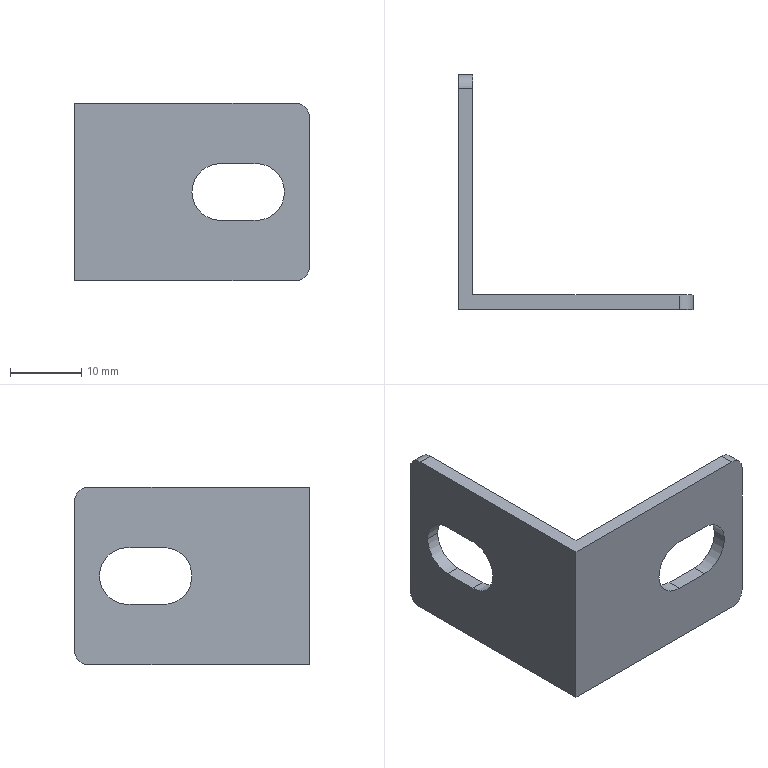Part | SolidWorks | features ICE 2, Extrusion 1, Fillet 1 | 1 solid | 22 faces | box 33 x 33 x 25 mm | volume 2832 mm3 | plane 12 | cylinder 10 | commonest cylinder face diameters 8 x6 4 x4
STEP:
#1=CARTESIAN_POINT('',(0.,29.5,12.5));
#2=VERTEX_POINT('',#1);
#3=CARTESIAN_POINT('',(0.,25.5,16.5));
#4=VERTEX_POINT('',#3);
#5=CARTESIAN_POINT('',(0.,25.5,12.5));
#6=DIRECTION('',(1.,0.,0.));
#7=DIRECTION('',(0.,1.,0.));
#8=AXIS2_PLACEMENT_3D('',#5,#6,#7);
#9=CIRCLE('',#8,4.);
#10=EDGE_CURVE('',#2,#4,#9,.T.);
#11=ORIENTED_EDGE('',*,*,#10,.F.);
#12=CARTESIAN_POINT('',(2.,29.5,12.5));
#13=VERTEX_POINT('',#12);
#14=CARTESIAN_POINT('',(0.,29.5,12.5));
#15=DIRECTION('',(1.,0.,0.));
#16=VECTOR('',#15,1000.);
#17=LINE('',#14,#16);
#18=EDGE_CURVE('',#2,#13,#17,.T.);
#19=ORIENTED_EDGE('',*,*,#18,.T.);
#20=CARTESIAN_POINT('',(2.,25.5,16.5));
#21=VERTEX_POINT('',#20);
#22=CARTESIAN_POINT('',(2.,25.5,12.5));
#23=DIRECTION('',(1.,0.,0.));
#24=DIRECTION('',(0.,1.,0.));
#25=AXIS2_PLACEMENT_3D('',#22,#23,#24);
#26=CIRCLE('',#25,4.);
#27=EDGE_CURVE('',#13,#21,#26,.T.);
#28=ORIENTED_EDGE('',*,*,#27,.T.);
#29=CARTESIAN_POINT('',(0.,25.5,16.5));
#30=DIRECTION('',(1.,0.,0.));
#31=VECTOR('',#30,1000.);
#32=LINE('',#29,#31);
#33=EDGE_CURVE('',#4,#21,#32,.T.);
#34=ORIENTED_EDGE('',*,*,#33,.F.);
#35=EDGE_LOOP('',(#11,#19,#28,#34));
#36=FACE_OUTER_BOUND('',#35,.T.);
#37=CARTESIAN_POINT('',(0.,25.5,12.5));
#38=DIRECTION('',(1.,0.,0.));
#39=DIRECTION('',(0.,1.,0.));
#40=AXIS2_PLACEMENT_3D('',#37,#38,#39);
#41=CYLINDRICAL_SURFACE('',#40,4.);
#42=ADVANCED_FACE('',(#36),#41,.F.);
#43=CARTESIAN_POINT('',(16.5,0.,12.5));
#44=VERTEX_POINT('',#43);
#45=CARTESIAN_POINT('',(20.5,0.,16.5));
#46=VERTEX_POINT('',#45);
#47=CARTESIAN_POINT('',(20.5,0.,12.5));
#48=DIRECTION('',(0.,1.,0.));
#49=DIRECTION('',(-1.,0.,0.));
#50=AXIS2_PLACEMENT_3D('',#47,#48,#49);
#51=CIRCLE('',#50,4.);
#52=EDGE_CURVE('',#44,#46,#51,.T.);
#53=ORIENTED_EDGE('',*,*,#52,.F.);
#54=CARTESIAN_POINT('',(16.5,2.,12.5));
#55=VERTEX_POINT('',#54);
#56=CARTESIAN_POINT('',(16.5,0.,12.5));
#57=DIRECTION('',(0.,1.,0.));
#58=VECTOR('',#57,1000.);
#59=LINE('',#56,#58);
#60=EDGE_CURVE('',#44,#55,#59,.T.);
#61=ORIENTED_EDGE('',*,*,#60,.T.);
#62=CARTESIAN_POINT('',(20.5,2.,16.5));
#63=VERTEX_POINT('',#62);
#64=CARTESIAN_POINT('',(20.5,2.,12.5));
#65=DIRECTION('',(0.,1.,0.));
#66=DIRECTION('',(-1.,0.,0.));
#67=AXIS2_PLACEMENT_3D('',#64,#65,#66);
#68=CIRCLE('',#67,4.);
#69=EDGE_CURVE('',#55,#63,#68,.T.);
#70=ORIENTED_EDGE('',*,*,#69,.T.);
#71=CARTESIAN_POINT('',(20.5,0.,16.5));
#72=DIRECTION('',(0.,1.,0.));
#73=VECTOR('',#72,1000.);
#74=LINE('',#71,#73);
#75=EDGE_CURVE('',#46,#63,#74,.T.);
#76=ORIENTED_EDGE('',*,*,#75,.F.);
#77=EDGE_LOOP('',(#53,#61,#70,#76));
#78=FACE_OUTER_BOUND('',#77,.T.);
#79=CARTESIAN_POINT('',(20.5,0.,12.5));
#80=DIRECTION('',(0.,1.,0.));
#81=DIRECTION('',(-1.,0.,0.));
#82=AXIS2_PLACEMENT_3D('',#79,#80,#81);
#83=CYLINDRICAL_SURFACE('',#82,4.);
#84=ADVANCED_FACE('',(#78),#83,.F.);
#85=CARTESIAN_POINT('',(0.,20.5,8.5));
#86=VERTEX_POINT('',#85);
#87=CARTESIAN_POINT('',(0.,25.5,8.5));
#88=VERTEX_POINT('',#87);
#89=CARTESIAN_POINT('',(0.,25.5,8.5));
#90=DIRECTION('',(0.,1.,0.));
#91=VECTOR('',#90,1000.);
#92=LINE('',#89,#91);
#93=EDGE_CURVE('',#86,#88,#92,.T.);
#94=ORIENTED_EDGE('',*,*,#93,.T.);
#95=CARTESIAN_POINT('',(0.,25.5,12.5));
#96=DIRECTION('',(1.,0.,0.));
#97=DIRECTION('',(0.,1.,0.));
#98=AXIS2_PLACEMENT_3D('',#95,#96,#97);
#99=CIRCLE('',#98,4.);
#100=EDGE_CURVE('',#88,#2,#99,.T.);
#101=ORIENTED_EDGE('',*,*,#100,.T.);
#102=ORIENTED_EDGE('',*,*,#10,.T.);
#103=CARTESIAN_POINT('',(0.,20.5,16.5));
#104=VERTEX_POINT('',#103);
#105=CARTESIAN_POINT('',(0.,25.5,16.5));
#106=DIRECTION('',(0.,-1.,0.));
#107=VECTOR('',#106,1000.);
#108=LINE('',#105,#107);
#109=EDGE_CURVE('',#4,#104,#108,.T.);
#110=ORIENTED_EDGE('',*,*,#109,.T.);
#111=CARTESIAN_POINT('',(0.,20.5,12.5));
#112=DIRECTION('',(1.,0.,0.));
#113=DIRECTION('',(0.,1.,0.));
#114=AXIS2_PLACEMENT_3D('',#111,#112,#113);
#115=CIRCLE('',#114,4.);
#116=EDGE_CURVE('',#104,#86,#115,.T.);
#117=ORIENTED_EDGE('',*,*,#116,.T.);
#118=EDGE_LOOP('',(#94,#101,#102,#110,#117));
#119=FACE_BOUND('',#118,.T.);
#120=CARTESIAN_POINT('',(0.,33.,23.));
#121=VERTEX_POINT('',#120);
#122=CARTESIAN_POINT('',(0.,33.,2.));
#123=VERTEX_POINT('',#122);
#124=CARTESIAN_POINT('',(0.,33.,25.));
#125=DIRECTION('',(0.,0.,-1.));
#126=VECTOR('',#125,1000.);
#127=LINE('',#124,#126);
#128=EDGE_CURVE('',#121,#123,#127,.T.);
#129=ORIENTED_EDGE('',*,*,#128,.T.);
#130=CARTESIAN_POINT('',(0.,31.,0.));
#131=VERTEX_POINT('',#130);
#132=CARTESIAN_POINT('',(0.,31.,2.));
#133=DIRECTION('',(-1.,0.,0.));
#134=DIRECTION('',(0.,1.,0.));
#135=AXIS2_PLACEMENT_3D('',#132,#133,#134);
#136=CIRCLE('',#135,2.);
#137=EDGE_CURVE('',#123,#131,#136,.T.);
#138=ORIENTED_EDGE('',*,*,#137,.T.);
#139=CARTESIAN_POINT('',(0.,0.,0.));
#140=VERTEX_POINT('',#139);
#141=CARTESIAN_POINT('',(0.,33.,0.));
#142=DIRECTION('',(0.,-1.,0.));
#143=VECTOR('',#142,1000.);
#144=LINE('',#141,#143);
#145=EDGE_CURVE('',#131,#140,#144,.T.);
#146=ORIENTED_EDGE('',*,*,#145,.T.);
#147=CARTESIAN_POINT('',(0.,0.,25.));
#148=VERTEX_POINT('',#147);
#149=CARTESIAN_POINT('',(0.,0.,25.));
#150=DIRECTION('',(0.,0.,-1.));
#151=VECTOR('',#150,1000.);
#152=LINE('',#149,#151);
#153=EDGE_CURVE('',#148,#140,#152,.T.);
#154=ORIENTED_EDGE('',*,*,#153,.F.);
#155=CARTESIAN_POINT('',(0.,31.,25.));
#156=VERTEX_POINT('',#155);
#157=CARTESIAN_POINT('',(0.,33.,25.));
#158=DIRECTION('',(0.,-1.,0.));
#159=VECTOR('',#158,1000.);
#160=LINE('',#157,#159);
#161=EDGE_CURVE('',#156,#148,#160,.T.);
#162=ORIENTED_EDGE('',*,*,#161,.F.);
#163=CARTESIAN_POINT('',(0.,31.,23.));
#164=DIRECTION('',(-1.,0.,0.));
#165=DIRECTION('',(0.,1.,0.));
#166=AXIS2_PLACEMENT_3D('',#163,#164,#165);
#167=CIRCLE('',#166,2.);
#168=EDGE_CURVE('',#156,#121,#167,.T.);
#169=ORIENTED_EDGE('',*,*,#168,.T.);
#170=EDGE_LOOP('',(#129,#138,#146,#154,#162,#169));
#171=FACE_OUTER_BOUND('',#170,.T.);
#172=CARTESIAN_POINT('',(0.,33.,25.));
#173=DIRECTION('',(1.,0.,0.));
#174=DIRECTION('',(0.,1.,0.));
#175=AXIS2_PLACEMENT_3D('',#172,#173,#174);
#176=PLANE('',#175);
#177=ADVANCED_FACE('',(#119,#171),#176,.F.);
#178=CARTESIAN_POINT('',(25.5,0.,8.5));
#179=VERTEX_POINT('',#178);
#180=CARTESIAN_POINT('',(20.5,0.,8.5));
#181=VERTEX_POINT('',#180);
#182=CARTESIAN_POINT('',(20.5,0.,8.5));
#183=DIRECTION('',(-1.,0.,0.));
#184=VECTOR('',#183,1000.);
#185=LINE('',#182,#184);
#186=EDGE_CURVE('',#179,#181,#185,.T.);
#187=ORIENTED_EDGE('',*,*,#186,.T.);
#188=CARTESIAN_POINT('',(20.5,0.,12.5));
#189=DIRECTION('',(0.,1.,0.));
#190=DIRECTION('',(-1.,0.,0.));
#191=AXIS2_PLACEMENT_3D('',#188,#189,#190);
#192=CIRCLE('',#191,4.);
#193=EDGE_CURVE('',#181,#44,#192,.T.);
#194=ORIENTED_EDGE('',*,*,#193,.T.);
#195=ORIENTED_EDGE('',*,*,#52,.T.);
#196=CARTESIAN_POINT('',(25.5,0.,16.5));
#197=VERTEX_POINT('',#196);
#198=CARTESIAN_POINT('',(20.5,0.,16.5));
#199=DIRECTION('',(1.,0.,0.));
#200=VECTOR('',#199,1000.);
#201=LINE('',#198,#200);
#202=EDGE_CURVE('',#46,#197,#201,.T.);
#203=ORIENTED_EDGE('',*,*,#202,.T.);
#204=CARTESIAN_POINT('',(25.5,0.,12.5));
#205=DIRECTION('',(0.,1.,0.));
#206=DIRECTION('',(-1.,0.,0.));
#207=AXIS2_PLACEMENT_3D('',#204,#205,#206);
#208=CIRCLE('',#207,4.);
#209=EDGE_CURVE('',#197,#179,#208,.T.);
#210=ORIENTED_EDGE('',*,*,#209,.T.);
#211=EDGE_LOOP('',(#187,#194,#195,#203,#210));
#212=FACE_BOUND('',#211,.T.);
#213=CARTESIAN_POINT('',(33.,0.,23.));
#214=VERTEX_POINT('',#213);
#215=CARTESIAN_POINT('',(33.,0.,2.));
#216=VERTEX_POINT('',#215);
#217=CARTESIAN_POINT('',(33.,0.,25.));
#218=DIRECTION('',(0.,0.,-1.));
#219=VECTOR('',#218,1000.);
#220=LINE('',#217,#219);
#221=EDGE_CURVE('',#214,#216,#220,.T.);
#222=ORIENTED_EDGE('',*,*,#221,.F.);
#223=CARTESIAN_POINT('',(31.,0.,25.));
#224=VERTEX_POINT('',#223);
#225=CARTESIAN_POINT('',(31.,0.,23.));
#226=DIRECTION('',(0.,-1.,0.));
#227=DIRECTION('',(0.,0.,1.));
#228=AXIS2_PLACEMENT_3D('',#225,#226,#227);
#229=CIRCLE('',#228,2.);
#230=EDGE_CURVE('',#214,#224,#229,.T.);
#231=ORIENTED_EDGE('',*,*,#230,.T.);
#232=CARTESIAN_POINT('',(0.,0.,25.));
#233=DIRECTION('',(1.,0.,0.));
#234=VECTOR('',#233,1000.);
#235=LINE('',#232,#234);
#236=EDGE_CURVE('',#148,#224,#235,.T.);
#237=ORIENTED_EDGE('',*,*,#236,.F.);
#238=ORIENTED_EDGE('',*,*,#153,.T.);
#239=CARTESIAN_POINT('',(31.,0.,0.));
#240=VERTEX_POINT('',#239);
#241=CARTESIAN_POINT('',(0.,0.,0.));
#242=DIRECTION('',(1.,0.,0.));
#243=VECTOR('',#242,1000.);
#244=LINE('',#241,#243);
#245=EDGE_CURVE('',#140,#240,#244,.T.);
#246=ORIENTED_EDGE('',*,*,#245,.T.);
#247=CARTESIAN_POINT('',(31.,0.,2.));
#248=DIRECTION('',(0.,-1.,0.));
#249=DIRECTION('',(0.,0.,1.));
#250=AXIS2_PLACEMENT_3D('',#247,#248,#249);
#251=CIRCLE('',#250,2.);
#252=EDGE_CURVE('',#240,#216,#251,.T.);
#253=ORIENTED_EDGE('',*,*,#252,.T.);
#254=EDGE_LOOP('',(#222,#231,#237,#238,#246,#253));
#255=FACE_OUTER_BOUND('',#254,.T.);
#256=CARTESIAN_POINT('',(0.,0.,25.));
#257=DIRECTION('',(0.,1.,0.));
#258=DIRECTION('',(0.,0.,1.));
#259=AXIS2_PLACEMENT_3D('',#256,#257,#258);
#260=PLANE('',#259);
#261=ADVANCED_FACE('',(#212,#255),#260,.F.);
#262=CARTESIAN_POINT('',(33.,2.,23.));
#263=VERTEX_POINT('',#262);
#264=CARTESIAN_POINT('',(33.,2.,2.));
#265=VERTEX_POINT('',#264);
#266=CARTESIAN_POINT('',(33.,2.,25.));
#267=DIRECTION('',(0.,0.,-1.));
#268=VECTOR('',#267,1000.);
#269=LINE('',#266,#268);
#270=EDGE_CURVE('',#263,#265,#269,.T.);
#271=ORIENTED_EDGE('',*,*,#270,.F.);
#272=CARTESIAN_POINT('',(33.,0.,23.));
#273=DIRECTION('',(0.,-1.,0.));
#274=VECTOR('',#273,1000.);
#275=LINE('',#272,#274);
#276=EDGE_CURVE('',#263,#214,#275,.T.);
#277=ORIENTED_EDGE('',*,*,#276,.T.);
#278=ORIENTED_EDGE('',*,*,#221,.T.);
#279=CARTESIAN_POINT('',(33.,0.,2.));
#280=DIRECTION('',(0.,1.,0.));
#281=VECTOR('',#280,1000.);
#282=LINE('',#279,#281);
#283=EDGE_CURVE('',#216,#265,#282,.T.);
#284=ORIENTED_EDGE('',*,*,#283,.T.);
#285=EDGE_LOOP('',(#271,#277,#278,#284));
#286=FACE_OUTER_BOUND('',#285,.T.);
#287=CARTESIAN_POINT('',(33.,0.,25.));
#288=DIRECTION('',(-1.,0.,0.));
#289=DIRECTION('',(0.,0.,1.));
#290=AXIS2_PLACEMENT_3D('',#287,#288,#289);
#291=PLANE('',#290);
#292=ADVANCED_FACE('',(#286),#291,.F.);
#293=CARTESIAN_POINT('',(25.5,2.,16.5));
#294=VERTEX_POINT('',#293);
#295=CARTESIAN_POINT('',(20.5,2.,16.5));
#296=DIRECTION('',(1.,0.,0.));
#297=VECTOR('',#296,1000.);
#298=LINE('',#295,#297);
#299=EDGE_CURVE('',#63,#294,#298,.T.);
#300=ORIENTED_EDGE('',*,*,#299,.F.);
#301=ORIENTED_EDGE('',*,*,#69,.F.);
#302=CARTESIAN_POINT('',(20.5,2.,8.5));
#303=VERTEX_POINT('',#302);
#304=CARTESIAN_POINT('',(20.5,2.,12.5));
#305=DIRECTION('',(0.,1.,0.));
#306=DIRECTION('',(-1.,0.,0.));
#307=AXIS2_PLACEMENT_3D('',#304,#305,#306);
#308=CIRCLE('',#307,4.);
#309=EDGE_CURVE('',#303,#55,#308,.T.);
#310=ORIENTED_EDGE('',*,*,#309,.F.);
#311=CARTESIAN_POINT('',(25.5,2.,8.5));
#312=VERTEX_POINT('',#311);
#313=CARTESIAN_POINT('',(20.5,2.,8.5));
#314=DIRECTION('',(-1.,0.,0.));
#315=VECTOR('',#314,1000.);
#316=LINE('',#313,#315);
#317=EDGE_CURVE('',#312,#303,#316,.T.);
#318=ORIENTED_EDGE('',*,*,#317,.F.);
#319=CARTESIAN_POINT('',(25.5,2.,12.5));
#320=DIRECTION('',(0.,1.,0.));
#321=DIRECTION('',(-1.,0.,0.));
#322=AXIS2_PLACEMENT_3D('',#319,#320,#321);
#323=CIRCLE('',#322,4.);
#324=EDGE_CURVE('',#294,#312,#323,.T.);
#325=ORIENTED_EDGE('',*,*,#324,.F.);
#326=EDGE_LOOP('',(#300,#301,#310,#318,#325));
#327=FACE_BOUND('',#326,.T.);
#328=CARTESIAN_POINT('',(31.,2.,25.));
#329=VERTEX_POINT('',#328);
#330=CARTESIAN_POINT('',(2.,2.,25.));
#331=VERTEX_POINT('',#330);
#332=CARTESIAN_POINT('',(33.,2.,25.));
#333=DIRECTION('',(-1.,0.,0.));
#334=VECTOR('',#333,1000.);
#335=LINE('',#332,#334);
#336=EDGE_CURVE('',#329,#331,#335,.T.);
#337=ORIENTED_EDGE('',*,*,#336,.F.);
#338=CARTESIAN_POINT('',(31.,2.,23.));
#339=DIRECTION('',(0.,1.,0.));
#340=DIRECTION('',(1.,0.,0.));
#341=AXIS2_PLACEMENT_3D('',#338,#339,#340);
#342=CIRCLE('',#341,2.);
#343=EDGE_CURVE('',#329,#263,#342,.T.);
#344=ORIENTED_EDGE('',*,*,#343,.T.);
#345=ORIENTED_EDGE('',*,*,#270,.T.);
#346=CARTESIAN_POINT('',(31.,2.,0.));
#347=VERTEX_POINT('',#346);
#348=CARTESIAN_POINT('',(31.,2.,2.));
#349=DIRECTION('',(0.,1.,0.));
#350=DIRECTION('',(1.,0.,0.));
#351=AXIS2_PLACEMENT_3D('',#348,#349,#350);
#352=CIRCLE('',#351,2.);
#353=EDGE_CURVE('',#265,#347,#352,.T.);
#354=ORIENTED_EDGE('',*,*,#353,.T.);
#355=CARTESIAN_POINT('',(2.,2.,0.));
#356=VERTEX_POINT('',#355);
#357=CARTESIAN_POINT('',(33.,2.,0.));
#358=DIRECTION('',(-1.,0.,0.));
#359=VECTOR('',#358,1000.);
#360=LINE('',#357,#359);
#361=EDGE_CURVE('',#347,#356,#360,.T.);
#362=ORIENTED_EDGE('',*,*,#361,.T.);
#363=CARTESIAN_POINT('',(2.,2.,25.));
#364=DIRECTION('',(0.,0.,-1.));
#365=VECTOR('',#364,1000.);
#366=LINE('',#363,#365);
#367=EDGE_CURVE('',#331,#356,#366,.T.);
#368=ORIENTED_EDGE('',*,*,#367,.F.);
#369=EDGE_LOOP('',(#337,#344,#345,#354,#362,#368));
#370=FACE_OUTER_BOUND('',#369,.T.);
#371=CARTESIAN_POINT('',(33.,2.,25.));
#372=DIRECTION('',(0.,-1.,0.));
#373=DIRECTION('',(1.,0.,0.));
#374=AXIS2_PLACEMENT_3D('',#371,#372,#373);
#375=PLANE('',#374);
#376=ADVANCED_FACE('',(#327,#370),#375,.F.);
#377=CARTESIAN_POINT('',(2.,20.5,16.5));
#378=VERTEX_POINT('',#377);
#379=CARTESIAN_POINT('',(2.,25.5,16.5));
#380=DIRECTION('',(0.,-1.,0.));
#381=VECTOR('',#380,1000.);
#382=LINE('',#379,#381);
#383=EDGE_CURVE('',#21,#378,#382,.T.);
#384=ORIENTED_EDGE('',*,*,#383,.F.);
#385=ORIENTED_EDGE('',*,*,#27,.F.);
#386=CARTESIAN_POINT('',(2.,25.5,8.5));
#387=VERTEX_POINT('',#386);
#388=CARTESIAN_POINT('',(2.,25.5,12.5));
#389=DIRECTION('',(1.,0.,0.));
#390=DIRECTION('',(0.,1.,0.));
#391=AXIS2_PLACEMENT_3D('',#388,#389,#390);
#392=CIRCLE('',#391,4.);
#393=EDGE_CURVE('',#387,#13,#392,.T.);
#394=ORIENTED_EDGE('',*,*,#393,.F.);
#395=CARTESIAN_POINT('',(2.,20.5,8.5));
#396=VERTEX_POINT('',#395);
#397=CARTESIAN_POINT('',(2.,25.5,8.5));
#398=DIRECTION('',(0.,1.,0.));
#399=VECTOR('',#398,1000.);
#400=LINE('',#397,#399);
#401=EDGE_CURVE('',#396,#387,#400,.T.);
#402=ORIENTED_EDGE('',*,*,#401,.F.);
#403=CARTESIAN_POINT('',(2.,20.5,12.5));
#404=DIRECTION('',(1.,0.,0.));
#405=DIRECTION('',(0.,1.,0.));
#406=AXIS2_PLACEMENT_3D('',#403,#404,#405);
#407=CIRCLE('',#406,4.);
#408=EDGE_CURVE('',#378,#396,#407,.T.);
#409=ORIENTED_EDGE('',*,*,#408,.F.);
#410=EDGE_LOOP('',(#384,#385,#394,#402,#409));
#411=FACE_BOUND('',#410,.T.);
#412=CARTESIAN_POINT('',(2.,31.,0.));
#413=VERTEX_POINT('',#412);
#414=CARTESIAN_POINT('',(2.,2.,0.));
#415=DIRECTION('',(0.,1.,0.));
#416=VECTOR('',#415,1000.);
#417=LINE('',#414,#416);
#418=EDGE_CURVE('',#356,#413,#417,.T.);
#419=ORIENTED_EDGE('',*,*,#418,.T.);
#420=CARTESIAN_POINT('',(2.,33.,2.));
#421=VERTEX_POINT('',#420);
#422=CARTESIAN_POINT('',(2.,31.,2.));
#423=DIRECTION('',(1.,0.,0.));
#424=DIRECTION('',(0.,-1.,0.));
#425=AXIS2_PLACEMENT_3D('',#422,#423,#424);
#426=CIRCLE('',#425,2.);
#427=EDGE_CURVE('',#413,#421,#426,.T.);
#428=ORIENTED_EDGE('',*,*,#427,.T.);
#429=CARTESIAN_POINT('',(2.,33.,23.));
#430=VERTEX_POINT('',#429);
#431=CARTESIAN_POINT('',(2.,33.,25.));
#432=DIRECTION('',(0.,0.,-1.));
#433=VECTOR('',#432,1000.);
#434=LINE('',#431,#433);
#435=EDGE_CURVE('',#430,#421,#434,.T.);
#436=ORIENTED_EDGE('',*,*,#435,.F.);
#437=CARTESIAN_POINT('',(2.,31.,25.));
#438=VERTEX_POINT('',#437);
#439=CARTESIAN_POINT('',(2.,31.,23.));
#440=DIRECTION('',(1.,0.,0.));
#441=DIRECTION('',(0.,-1.,0.));
#442=AXIS2_PLACEMENT_3D('',#439,#440,#441);
#443=CIRCLE('',#442,2.);
#444=EDGE_CURVE('',#430,#438,#443,.T.);
#445=ORIENTED_EDGE('',*,*,#444,.T.);
#446=CARTESIAN_POINT('',(2.,2.,25.));
#447=DIRECTION('',(0.,1.,0.));
#448=VECTOR('',#447,1000.);
#449=LINE('',#446,#448);
#450=EDGE_CURVE('',#331,#438,#449,.T.);
#451=ORIENTED_EDGE('',*,*,#450,.F.);
#452=ORIENTED_EDGE('',*,*,#367,.T.);
#453=EDGE_LOOP('',(#419,#428,#436,#445,#451,#452));
#454=FACE_OUTER_BOUND('',#453,.T.);
#455=CARTESIAN_POINT('',(2.,2.,25.));
#456=DIRECTION('',(-1.,0.,0.));
#457=DIRECTION('',(0.,-1.,0.));
#458=AXIS2_PLACEMENT_3D('',#455,#456,#457);
#459=PLANE('',#458);
#460=ADVANCED_FACE('',(#411,#454),#459,.F.);
#461=ORIENTED_EDGE('',*,*,#435,.T.);
#462=CARTESIAN_POINT('',(2.,33.,2.));
#463=DIRECTION('',(-1.,0.,0.));
#464=VECTOR('',#463,1000.);
#465=LINE('',#462,#464);
#466=EDGE_CURVE('',#421,#123,#465,.T.);
#467=ORIENTED_EDGE('',*,*,#466,.T.);
#468=ORIENTED_EDGE('',*,*,#128,.F.);
#469=CARTESIAN_POINT('',(2.,33.,23.));
#470=DIRECTION('',(1.,0.,0.));
#471=VECTOR('',#470,1000.);
#472=LINE('',#469,#471);
#473=EDGE_CURVE('',#121,#430,#472,.T.);
#474=ORIENTED_EDGE('',*,*,#473,.T.);
#475=EDGE_LOOP('',(#461,#467,#468,#474));
#476=FACE_OUTER_BOUND('',#475,.T.);
#477=CARTESIAN_POINT('',(2.,33.,25.));
#478=DIRECTION('',(0.,-1.,0.));
#479=DIRECTION('',(0.,0.,-1.));
#480=AXIS2_PLACEMENT_3D('',#477,#478,#479);
#481=PLANE('',#480);
#482=ADVANCED_FACE('',(#476),#481,.F.);
#483=ORIENTED_EDGE('',*,*,#236,.T.);
#484=CARTESIAN_POINT('',(31.,2.,25.));
#485=DIRECTION('',(0.,1.,0.));
#486=VECTOR('',#485,1000.);
#487=LINE('',#484,#486);
#488=EDGE_CURVE('',#224,#329,#487,.T.);
#489=ORIENTED_EDGE('',*,*,#488,.T.);
#490=ORIENTED_EDGE('',*,*,#336,.T.);
#491=ORIENTED_EDGE('',*,*,#450,.T.);
#492=CARTESIAN_POINT('',(0.,31.,25.));
#493=DIRECTION('',(-1.,0.,0.));
#494=VECTOR('',#493,1000.);
#495=LINE('',#492,#494);
#496=EDGE_CURVE('',#438,#156,#495,.T.);
#497=ORIENTED_EDGE('',*,*,#496,.T.);
#498=ORIENTED_EDGE('',*,*,#161,.T.);
#499=EDGE_LOOP('',(#483,#489,#490,#491,#497,#498));
#500=FACE_OUTER_BOUND('',#499,.T.);
#501=CARTESIAN_POINT('',(0.,0.,25.));
#502=DIRECTION('',(0.,0.,1.));
#503=DIRECTION('',(1.,0.,0.));
#504=AXIS2_PLACEMENT_3D('',#501,#502,#503);
#505=PLANE('',#504);
#506=ADVANCED_FACE('',(#500),#505,.T.);
#507=ORIENTED_EDGE('',*,*,#361,.F.);
#508=CARTESIAN_POINT('',(31.,0.,0.));
#509=DIRECTION('',(0.,-1.,0.));
#510=VECTOR('',#509,1000.);
#511=LINE('',#508,#510);
#512=EDGE_CURVE('',#347,#240,#511,.T.);
#513=ORIENTED_EDGE('',*,*,#512,.T.);
#514=ORIENTED_EDGE('',*,*,#245,.F.);
#515=ORIENTED_EDGE('',*,*,#145,.F.);
#516=CARTESIAN_POINT('',(0.,31.,0.));
#517=DIRECTION('',(1.,0.,0.));
#518=VECTOR('',#517,1000.);
#519=LINE('',#516,#518);
#520=EDGE_CURVE('',#131,#413,#519,.T.);
#521=ORIENTED_EDGE('',*,*,#520,.T.);
#522=ORIENTED_EDGE('',*,*,#418,.F.);
#523=EDGE_LOOP('',(#507,#513,#514,#515,#521,#522));
#524=FACE_OUTER_BOUND('',#523,.T.);
#525=CARTESIAN_POINT('',(0.,0.,0.));
#526=DIRECTION('',(0.,0.,1.));
#527=DIRECTION('',(1.,0.,0.));
#528=AXIS2_PLACEMENT_3D('',#525,#526,#527);
#529=PLANE('',#528);
#530=ADVANCED_FACE('',(#524),#529,.F.);
#531=ORIENTED_EDGE('',*,*,#230,.F.);
#532=ORIENTED_EDGE('',*,*,#276,.F.);
#533=ORIENTED_EDGE('',*,*,#343,.F.);
#534=ORIENTED_EDGE('',*,*,#488,.F.);
#535=EDGE_LOOP('',(#531,#532,#533,#534));
#536=FACE_OUTER_BOUND('',#535,.T.);
#537=CARTESIAN_POINT('',(31.,0.,23.));
#538=DIRECTION('',(0.,-1.,0.));
#539=DIRECTION('',(0.,0.,-1.));
#540=AXIS2_PLACEMENT_3D('',#537,#538,#539);
#541=CYLINDRICAL_SURFACE('',#540,2.);
#542=ADVANCED_FACE('',(#536),#541,.T.);
#543=ORIENTED_EDGE('',*,*,#252,.F.);
#544=ORIENTED_EDGE('',*,*,#512,.F.);
#545=ORIENTED_EDGE('',*,*,#353,.F.);
#546=ORIENTED_EDGE('',*,*,#283,.F.);
#547=EDGE_LOOP('',(#543,#544,#545,#546));
#548=FACE_OUTER_BOUND('',#547,.T.);
#549=CARTESIAN_POINT('',(31.,0.,2.));
#550=DIRECTION('',(0.,1.,0.));
#551=DIRECTION('',(0.,0.,1.));
#552=AXIS2_PLACEMENT_3D('',#549,#550,#551);
#553=CYLINDRICAL_SURFACE('',#552,2.);
#554=ADVANCED_FACE('',(#548),#553,.T.);
#555=ORIENTED_EDGE('',*,*,#427,.F.);
#556=ORIENTED_EDGE('',*,*,#520,.F.);
#557=ORIENTED_EDGE('',*,*,#137,.F.);
#558=ORIENTED_EDGE('',*,*,#466,.F.);
#559=EDGE_LOOP('',(#555,#556,#557,#558));
#560=FACE_OUTER_BOUND('',#559,.T.);
#561=CARTESIAN_POINT('',(2.,31.,2.));
#562=DIRECTION('',(-1.,0.,0.));
#563=DIRECTION('',(0.,0.,1.));
#564=AXIS2_PLACEMENT_3D('',#561,#562,#563);
#565=CYLINDRICAL_SURFACE('',#564,2.);
#566=ADVANCED_FACE('',(#560),#565,.T.);
#567=ORIENTED_EDGE('',*,*,#444,.F.);
#568=ORIENTED_EDGE('',*,*,#473,.F.);
#569=ORIENTED_EDGE('',*,*,#168,.F.);
#570=ORIENTED_EDGE('',*,*,#496,.F.);
#571=EDGE_LOOP('',(#567,#568,#569,#570));
#572=FACE_OUTER_BOUND('',#571,.T.);
#573=CARTESIAN_POINT('',(0.,31.,23.));
#574=DIRECTION('',(1.,0.,0.));
#575=DIRECTION('',(0.,0.,-1.));
#576=AXIS2_PLACEMENT_3D('',#573,#574,#575);
#577=CYLINDRICAL_SURFACE('',#576,2.);
#578=ADVANCED_FACE('',(#572),#577,.T.);
#579=ORIENTED_EDGE('',*,*,#60,.F.);
#580=ORIENTED_EDGE('',*,*,#193,.F.);
#581=CARTESIAN_POINT('',(20.5,0.,8.5));
#582=DIRECTION('',(0.,1.,0.));
#583=VECTOR('',#582,1000.);
#584=LINE('',#581,#583);
#585=EDGE_CURVE('',#181,#303,#584,.T.);
#586=ORIENTED_EDGE('',*,*,#585,.T.);
#587=ORIENTED_EDGE('',*,*,#309,.T.);
#588=EDGE_LOOP('',(#579,#580,#586,#587));
#589=FACE_OUTER_BOUND('',#588,.T.);
#590=CARTESIAN_POINT('',(20.5,0.,12.5));
#591=DIRECTION('',(0.,1.,0.));
#592=DIRECTION('',(-1.,0.,0.));
#593=AXIS2_PLACEMENT_3D('',#590,#591,#592);
#594=CYLINDRICAL_SURFACE('',#593,4.);
#595=ADVANCED_FACE('',(#589),#594,.F.);
#596=ORIENTED_EDGE('',*,*,#317,.T.);
#597=ORIENTED_EDGE('',*,*,#585,.F.);
#598=ORIENTED_EDGE('',*,*,#186,.F.);
#599=CARTESIAN_POINT('',(25.5,0.,8.5));
#600=DIRECTION('',(0.,1.,0.));
#601=VECTOR('',#600,1000.);
#602=LINE('',#599,#601);
#603=EDGE_CURVE('',#179,#312,#602,.T.);
#604=ORIENTED_EDGE('',*,*,#603,.T.);
#605=EDGE_LOOP('',(#596,#597,#598,#604));
#606=FACE_OUTER_BOUND('',#605,.T.);
#607=CARTESIAN_POINT('',(20.5,0.,8.5));
#608=DIRECTION('',(0.,0.,-1.));
#609=DIRECTION('',(-1.,0.,0.));
#610=AXIS2_PLACEMENT_3D('',#607,#608,#609);
#611=PLANE('',#610);
#612=ADVANCED_FACE('',(#606),#611,.F.);
#613=ORIENTED_EDGE('',*,*,#324,.T.);
#614=ORIENTED_EDGE('',*,*,#603,.F.);
#615=ORIENTED_EDGE('',*,*,#209,.F.);
#616=CARTESIAN_POINT('',(25.5,0.,16.5));
#617=DIRECTION('',(0.,1.,0.));
#618=VECTOR('',#617,1000.);
#619=LINE('',#616,#618);
#620=EDGE_CURVE('',#197,#294,#619,.T.);
#621=ORIENTED_EDGE('',*,*,#620,.T.);
#622=EDGE_LOOP('',(#613,#614,#615,#621));
#623=FACE_OUTER_BOUND('',#622,.T.);
#624=CARTESIAN_POINT('',(25.5,0.,12.5));
#625=DIRECTION('',(0.,1.,0.));
#626=DIRECTION('',(-1.,0.,0.));
#627=AXIS2_PLACEMENT_3D('',#624,#625,#626);
#628=CYLINDRICAL_SURFACE('',#627,4.);
#629=ADVANCED_FACE('',(#623),#628,.F.);
#630=ORIENTED_EDGE('',*,*,#299,.T.);
#631=ORIENTED_EDGE('',*,*,#620,.F.);
#632=ORIENTED_EDGE('',*,*,#202,.F.);
#633=ORIENTED_EDGE('',*,*,#75,.T.);
#634=EDGE_LOOP('',(#630,#631,#632,#633));
#635=FACE_OUTER_BOUND('',#634,.T.);
#636=CARTESIAN_POINT('',(20.5,0.,16.5));
#637=DIRECTION('',(0.,0.,1.));
#638=DIRECTION('',(1.,0.,0.));
#639=AXIS2_PLACEMENT_3D('',#636,#637,#638);
#640=PLANE('',#639);
#641=ADVANCED_FACE('',(#635),#640,.F.);
#642=ORIENTED_EDGE('',*,*,#18,.F.);
#643=ORIENTED_EDGE('',*,*,#100,.F.);
#644=CARTESIAN_POINT('',(0.,25.5,8.5));
#645=DIRECTION('',(1.,0.,0.));
#646=VECTOR('',#645,1000.);
#647=LINE('',#644,#646);
#648=EDGE_CURVE('',#88,#387,#647,.T.);
#649=ORIENTED_EDGE('',*,*,#648,.T.);
#650=ORIENTED_EDGE('',*,*,#393,.T.);
#651=EDGE_LOOP('',(#642,#643,#649,#650));
#652=FACE_OUTER_BOUND('',#651,.T.);
#653=CARTESIAN_POINT('',(0.,25.5,12.5));
#654=DIRECTION('',(1.,0.,0.));
#655=DIRECTION('',(0.,1.,0.));
#656=AXIS2_PLACEMENT_3D('',#653,#654,#655);
#657=CYLINDRICAL_SURFACE('',#656,4.);
#658=ADVANCED_FACE('',(#652),#657,.F.);
#659=ORIENTED_EDGE('',*,*,#401,.T.);
#660=ORIENTED_EDGE('',*,*,#648,.F.);
#661=ORIENTED_EDGE('',*,*,#93,.F.);
#662=CARTESIAN_POINT('',(0.,20.5,8.5));
#663=DIRECTION('',(1.,0.,0.));
#664=VECTOR('',#663,1000.);
#665=LINE('',#662,#664);
#666=EDGE_CURVE('',#86,#396,#665,.T.);
#667=ORIENTED_EDGE('',*,*,#666,.T.);
#668=EDGE_LOOP('',(#659,#660,#661,#667));
#669=FACE_OUTER_BOUND('',#668,.T.);
#670=CARTESIAN_POINT('',(0.,25.5,8.5));
#671=DIRECTION('',(0.,0.,-1.));
#672=DIRECTION('',(0.,1.,0.));
#673=AXIS2_PLACEMENT_3D('',#670,#671,#672);
#674=PLANE('',#673);
#675=ADVANCED_FACE('',(#669),#674,.F.);
#676=ORIENTED_EDGE('',*,*,#408,.T.);
#677=ORIENTED_EDGE('',*,*,#666,.F.);
#678=ORIENTED_EDGE('',*,*,#116,.F.);
#679=CARTESIAN_POINT('',(0.,20.5,16.5));
#680=DIRECTION('',(1.,0.,0.));
#681=VECTOR('',#680,1000.);
#682=LINE('',#679,#681);
#683=EDGE_CURVE('',#104,#378,#682,.T.);
#684=ORIENTED_EDGE('',*,*,#683,.T.);
#685=EDGE_LOOP('',(#676,#677,#678,#684));
#686=FACE_OUTER_BOUND('',#685,.T.);
#687=CARTESIAN_POINT('',(0.,20.5,12.5));
#688=DIRECTION('',(1.,0.,0.));
#689=DIRECTION('',(0.,1.,0.));
#690=AXIS2_PLACEMENT_3D('',#687,#688,#689);
#691=CYLINDRICAL_SURFACE('',#690,4.);
#692=ADVANCED_FACE('',(#686),#691,.F.);
#693=ORIENTED_EDGE('',*,*,#383,.T.);
#694=ORIENTED_EDGE('',*,*,#683,.F.);
#695=ORIENTED_EDGE('',*,*,#109,.F.);
#696=ORIENTED_EDGE('',*,*,#33,.T.);
#697=EDGE_LOOP('',(#693,#694,#695,#696));
#698=FACE_OUTER_BOUND('',#697,.T.);
#699=CARTESIAN_POINT('',(0.,25.5,16.5));
#700=DIRECTION('',(0.,0.,1.));
#701=DIRECTION('',(1.,0.,0.));
#702=AXIS2_PLACEMENT_3D('',#699,#700,#701);
#703=PLANE('',#702);
#704=ADVANCED_FACE('',(#698),#703,.F.);
#705=CLOSED_SHELL('',(#42,#84,#177,#261,#292,#376,#460,#482,#506,#530,#542,#554,#566,#578,#595,#612,#629,#641,#658,#675,#692,#704));
#706=MANIFOLD_SOLID_BREP('',#705);
#707=CARTESIAN_POINT('',(0.,0.,0.));
#708=DIRECTION('',(0.,0.,1.));
#709=DIRECTION('',(1.,0.,0.));
#710=AXIS2_PLACEMENT_3D('',#707,#708,#709);
#711=(LENGTH_UNIT()NAMED_UNIT(*)SI_UNIT(.MILLI.,.METRE.));
#712=UNCERTAINTY_MEASURE_WITH_UNIT(LENGTH_MEASURE(0.00001),#711,'','');
#713=(NAMED_UNIT(*)PLANE_ANGLE_UNIT()SI_UNIT($,.RADIAN.));
#714=(NAMED_UNIT(*)SI_UNIT($,.STERADIAN.)SOLID_ANGLE_UNIT());
#715=(GEOMETRIC_REPRESENTATION_CONTEXT(3)GLOBAL_UNCERTAINTY_ASSIGNED_CONTEXT((#712))GLOBAL_UNIT_ASSIGNED_CONTEXT((#711,#713,#714))REPRESENTATION_CONTEXT('',''));
#716=ADVANCED_BREP_SHAPE_REPRESENTATION('',(#706,#710),#715);